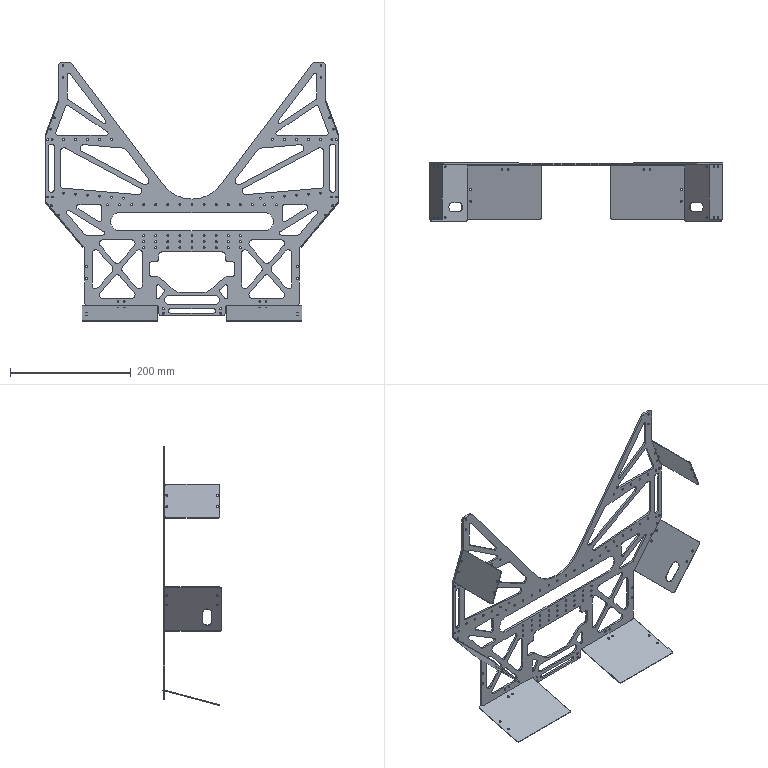Part | SolidWorks | features ICE 8, Fillet 4, Extrusion 1, MirrorSolid 1 | 7 solids | 547 faces | box 486 x 96.259 x 428.466 mm | volume 244289 mm3 | cylinder 398 | plane 149 | commonest cylinder face diameters 3.2 x240 6 x62 12 x46 8 x22 10 x10 15 x6